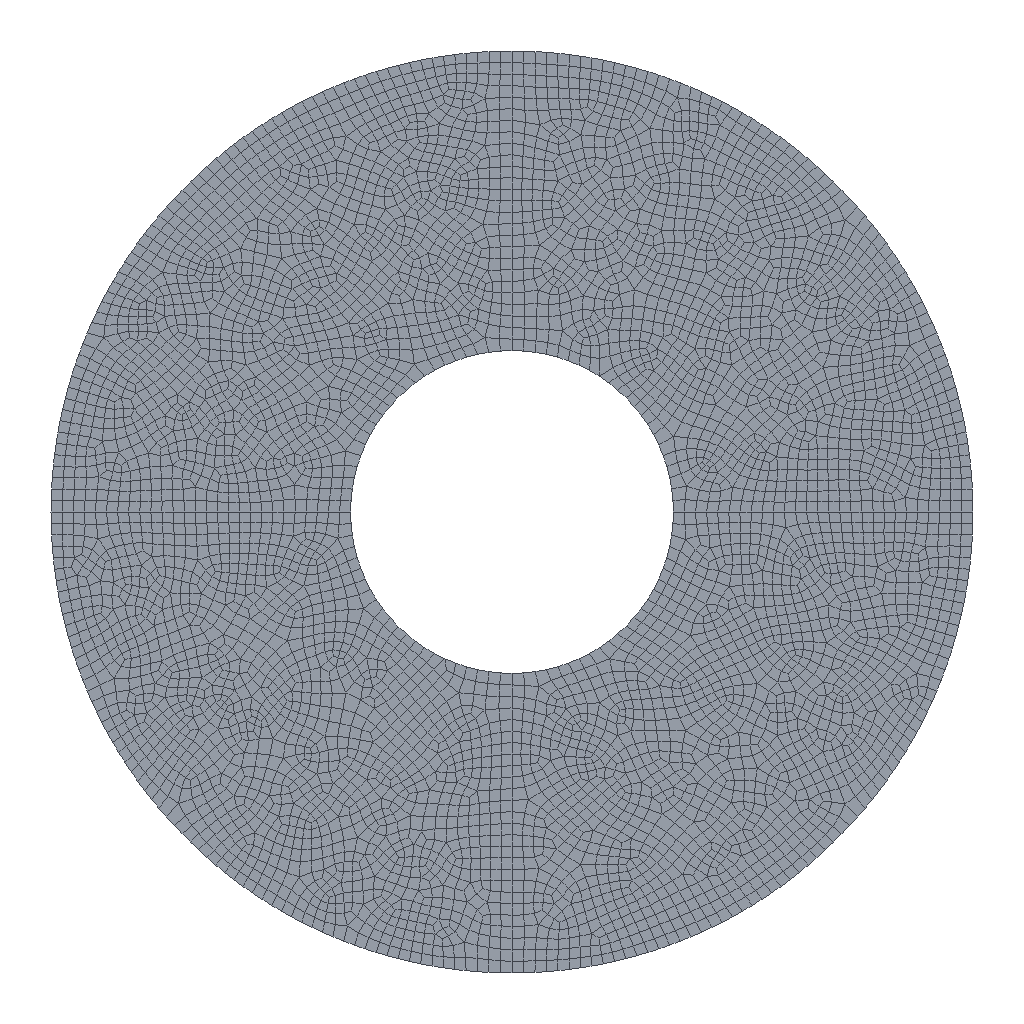Simulation study | abaqus
Set-up summary:
category,name,step,type,value,unit,region
solver,abaqus
solver,version,,,Abaqus/Standard 2020
units,not stated in the deck,,not stated
analysis,deck,,geostatic,geostatic; soils
load_step,Step-1,Step-1,geostatic,nlgeom=False
load_step,Step-2,Step-2,soils,nlgeom=True
contact,interactions,,,general=0 pairs=0 ties=0
load_step,requested,,,2
mesh,nodes,,,5893
mesh,elements,,,5609
element_type,CPE4RP,,plane,5503
element_type,COH2D4P,,cohesive,106
load,load commands in deck,,count,4
bc,support commands in deck,,count,2
material,BASE,,in results
material,MATERIAL-1,,in results
check,setup vs results,,match,"per instance, exact: element labels, types and connectivity; labels of the nodes the elements use; coordinates of those nodes at SINGLE_PRECISION in 1 of 1 instance(s)"
Abaqus input file, long lists of numbers shortened:
*Heading
** Job name: Job-1 Model name: Model-1
** Generated by: Abaqus/CAE 2020
*Preprint, echo=NO, model=NO, history=NO, contact=NO
**
** PARTS
**
*Part, name=Part-1
*Node
      1,           0.,         -20.
      2,           0.,          -7.
** (5891 more lines like these left out)
*Element, type=CPE4RP
   1,  141,  142,  707,  716
   2, 1011,  990,  980,  936
** (5501 more lines like these left out)
*Element, type=COH2D4P
5504, 5674, 5699,    8,  276, 5702, 5701
5505, 5675, 5674,  276,  275, 5703, 5702
** (104 more lines like these left out)
*Nset, nset=Set-19
    1,    2,    3,    4,    5,    6,    7,    8,    9,   10,   11,   12,   13,   14,   15,   16
   17,   18,   19,   20,   21,   22,   23,   24,   25,   26,   27,   28,   29,   30,   31,   32
** (360 more lines like these left out)
*Elset, elset=Set-19, generate
    1,  5503,     1
*Elset, elset=CohesiveSeam-2-Elements, generate
 5504,  5529,     1
*Nset, nset=CohesiveSeam-2-TopNodes
   7,   8, 252, 253, 254, 255, 256, 257, 258, 259, 260, 261, 262, 263, 264, 265
 266, 267, 268, 269, 270, 271, 272, 273, 274, 275, 276
*Nset, nset=CohesiveSeam-2-BottomNodes, generate
 5674,  5700,     1
*Nset, nset=CohesiveSeam-2-MidNodes, generate
 5701,  5727,     1
*Elset, elset=CohesiveSeam-3-Elements, generate
 5530,  5556,     1
*Nset, nset=CohesiveSeam-3-TopNodes
  3,  4, 55, 56, 57, 58, 59, 60, 61, 62, 63, 64, 65, 66, 67, 68
 69, 70, 71, 72, 73, 74, 75, 76, 77, 78, 79, 80
*Nset, nset=CohesiveSeam-3-BottomNodes, generate
 5728,  5755,     1
*Nset, nset=CohesiveSeam-3-MidNodes, generate
 5756,  5783,     1
*Elset, elset=CohesiveSeam-4-Elements, generate
 5557,  5582,     1
*Nset, nset=CohesiveSeam-4-TopNodes
  1,  2,  9, 10, 11, 12, 13, 14, 15, 16, 17, 18, 19, 20, 21, 22
 23, 24, 25, 26, 27, 28, 29, 30, 31, 32, 33
*Nset, nset=CohesiveSeam-4-BottomNodes, generate
 5784,  5810,     1
*Nset, nset=CohesiveSeam-4-MidNodes, generate
 5811,  5837,     1
*Elset, elset=CohesiveSeam-5-Elements, generate
 5583,  5609,     1
*Nset, nset=CohesiveSeam-5-TopNodes
   5,   6, 205, 206, 207, 208, 209, 210, 211, 212, 213, 214, 215, 216, 217, 218
 219, 220, 221, 222, 223, 224, 225, 226, 227, 228, 229, 230
*Nset, nset=CohesiveSeam-5-BottomNodes, generate
 5838,  5865,     1
*Nset, nset=CohesiveSeam-5-MidNodes, generate
 5866,  5893,     1
*Nset, nset=in2
 5727,
*Nset, nset=in3
 5783,
*Nset, nset=in4
 5811,
*Nset, nset=in5
 5866,
*Elset, elset=initial2, generate
 5526,  5529,     1
*Elset, elset=initial3, generate
 5553,  5556,     1
*Elset, elset=initial4, generate
 5557,  5560,     1
*Elset, elset=initial5, generate
 5583,  5585,     1
*Elset, elset=__PickedSurf7_S3, internal
   60,   75,   89,   90,  134,  149,  482,  483,  522, 5557, 5558, 5559, 5560, 5561, 5562, 5563
 5564, 5565, 5566, 5567, 5568, 5569, 5570, 5571, 5572, 5573, 5574, 5575, 5576, 5577, 5578, 5579
** (1 more lines like these left out)
*Elset, elset=__PickedSurf7_S1, internal
   55,   56,   57,  133,  151,  439,  480,  507,  509,  510,  511,  514,  516,  517,  518,  519
  524, 2829, 3207
*Elset, elset=__PickedSurf7_S4, internal
  470, 1561, 1565, 1583, 1599, 1600, 1875, 1877, 1879, 1880, 2795, 2826, 2845, 2851, 3209, 3213
 3214,
*Elset, elset=__PickedSurf7_S2, internal
 1495, 1497, 1512, 1523, 1560, 1584, 1585, 1874, 1890, 1892, 1893, 1895, 1898, 1900, 1903, 1905
 1907, 1908, 2776, 2797, 2808, 2825, 2830, 2849, 2850, 3309, 3311, 3313, 3315, 3318, 3319, 3320
** (1 more lines like these left out)
*Surface, type=ELEMENT, name=_PickedSurf7, internal
__PickedSurf7_S3, S3
__PickedSurf7_S1, S1
__PickedSurf7_S4, S4
__PickedSurf7_S2, S2
*Elset, elset=__PickedSurf19_S2, internal
 2776, 2797, 2808, 2825, 2830, 2849, 2850, 3309, 3311, 3313, 3315, 3318, 3319, 3320, 3321, 3324
 3326,
*Elset, elset=__PickedSurf19_S4, internal
 2795, 2826, 2845, 2851, 3209, 3213, 3214
*Elset, elset=__PickedSurf19_S1, internal
 2829, 3207
*Surface, type=ELEMENT, name=_PickedSurf19, internal
__PickedSurf19_S2, S2
__PickedSurf19_S4, S4
__PickedSurf19_S1, S1
*Elset, elset=__PickedSurf26_S1, internal
  55,  56,  57, 133, 151, 439, 480, 507, 509, 510, 511, 514, 516, 517, 518, 519
 524,
*Elset, elset=__PickedSurf26_S3, internal
  60,  75,  89,  90, 134, 149, 482, 483, 522
*Elset, elset=__PickedSurf26_S4, internal
 470,
*Surface, type=ELEMENT, name=_PickedSurf26, internal
__PickedSurf26_S1, S1
__PickedSurf26_S3, S3
__PickedSurf26_S4, S4
*Elset, elset=__PickedSurf33_S3, internal, generate
 5557,  5582,     1
*Surface, type=ELEMENT, name=_PickedSurf33, internal
__PickedSurf33_S3, S3
*Elset, elset=__PickedSurf40_S2, internal
 1495, 1497, 1512, 1523, 1560, 1584, 1585, 1874, 1890, 1892, 1893, 1895, 1898, 1900, 1903, 1905
 1907, 1908
*Elset, elset=__PickedSurf40_S4, internal
 1561, 1565, 1583, 1599, 1600, 1875, 1877, 1879, 1880
*Surface, type=ELEMENT, name=_PickedSurf40, internal
__PickedSurf40_S2, S2
__PickedSurf40_S4, S4
*Elset, elset=_CohesiveSeam-2-TopSurf_S3, internal, generate
 5504,  5529,     1
*Surface, type=ELEMENT, name=CohesiveSeam-2-TopSurf
_CohesiveSeam-2-TopSurf_S3, S3
*Elset, elset=_CohesiveSeam-2-BottomSurf_S1, internal, generate
 5504,  5529,     1
*Surface, type=ELEMENT, name=CohesiveSeam-2-BottomSurf
_CohesiveSeam-2-BottomSurf_S1, S1
*Elset, elset=_CohesiveSeam-3-TopSurf_S3, internal, generate
 5530,  5556,     1
*Surface, type=ELEMENT, name=CohesiveSeam-3-TopSurf
_CohesiveSeam-3-TopSurf_S3, S3
*Elset, elset=_CohesiveSeam-3-BottomSurf_S1, internal, generate
 5530,  5556,     1
*Surface, type=ELEMENT, name=CohesiveSeam-3-BottomSurf
_CohesiveSeam-3-BottomSurf_S1, S1
*Elset, elset=_CohesiveSeam-4-TopSurf_S3, internal, generate
 5557,  5582,     1
*Surface, type=ELEMENT, name=CohesiveSeam-4-TopSurf
_CohesiveSeam-4-TopSurf_S3, S3
*Elset, elset=_CohesiveSeam-4-BottomSurf_S1, internal, generate
 5557,  5582,     1
*Surface, type=ELEMENT, name=CohesiveSeam-4-BottomSurf
_CohesiveSeam-4-BottomSurf_S1, S1
*Elset, elset=_CohesiveSeam-5-TopSurf_S3, internal, generate
 5583,  5609,     1
*Surface, type=ELEMENT, name=CohesiveSeam-5-TopSurf
_CohesiveSeam-5-TopSurf_S3, S3
*Elset, elset=_CohesiveSeam-5-BottomSurf_S1, internal, generate
 5583,  5609,     1
*Surface, type=ELEMENT, name=CohesiveSeam-5-BottomSurf
_CohesiveSeam-5-BottomSurf_S1, S1
** Section: Section-base
*Solid Section, elset=Set-19, material=base
,
** Section: Section-coh
*Cohesive Section, elset=CohesiveSeam-2-Elements, controls=EC-1, material=Material-1, response=TRACTION SEPARATION
,
** Section: Section-coh
*Cohesive Section, elset=CohesiveSeam-3-Elements, controls=EC-1, material=Material-1, response=TRACTION SEPARATION
,
** Section: Section-coh
*Cohesive Section, elset=CohesiveSeam-4-Elements, controls=EC-1, material=Material-1, response=TRACTION SEPARATION
,
** Section: Section-coh
*Cohesive Section, elset=CohesiveSeam-5-Elements, controls=EC-1, material=Material-1, response=TRACTION SEPARATION
,
*End Part
**
**
** ASSEMBLY
**
*Assembly, name=Assembly
**
*Instance, name=Part-1-1, part=Part-1
*End Instance
**
*Nset, nset=Set-1, instance=Part-1-1
    1,    2,    3,    4,    5,    6,    7,    8,    9,   10,   11,   12,   13,   14,   15,   16
   17,   18,   19,   20,   21,   22,   23,   24,   25,   26,   27,   28,   29,   30,   31,   32
** (360 more lines like these left out)
*Elset, elset=Set-1, instance=Part-1-1, generate
    1,  5609,     1
*Nset, nset=Set-2, instance=Part-1-1
    1,    2,    3,    4,    5,    6,    7,    8,    9,   10,   11,   12,   13,   14,   15,   16
   17,   18,   19,   20,   21,   22,   23,   24,   25,   26,   27,   28,   29,   30,   31,   32
** (360 more lines like these left out)
*Elset, elset=Set-2, instance=Part-1-1, generate
    1,  5503,     1
*Nset, nset=Set-3, instance=Part-1-1
    1,    4,    5,    8,   81,   82,   83,   84,   85,   86,   87,   88,   89,   90,   91,   92
   93,   94,   95,   96,   97,   98,   99,  100,  101,  102,  103,  104,  105,  106,  107,  108
** (14 more lines like these left out)
*Elset, elset=Set-3, instance=Part-1-1
    1,   17,   33,   34,   35,  152,  166,  168,  169,  181,  182,  183,  184,  193,  194,  197
  200,  203,  207,  208,  209,  210,  211,  213,  214,  274,  308,  354,  464,  480,  487,  490
** (14 more lines like these left out)
*Nset, nset=Set-4, instance=Part-1-1
    2,    3,    6,    7,   34,   35,   36,   37,   38,   39,   40,   41,   42,   43,   44,   45
   46,   47,   48,   49,   50,   51,   52,   53,   54,  231,  232,  233,  234,  235,  236,  237
** (4 more lines like these left out)
*Elset, elset=Set-4, instance=Part-1-1
  101,  103,  118,  126,  127,  128,  130,  145,  423,  457,  465,  470,  471,  472,  473,  474
  475,  476,  477,  478,  479,  568, 1386, 1406, 1409, 1601, 1610, 1611, 1626, 1627, 1639, 1714
** (4 more lines like these left out)
*Nset, nset=Set-5, instance=Part-1-1
    1,    4,    5,    8,   81,   82,   83,   84,   85,   86,   87,   88,   89,   90,   91,   92
   93,   94,   95,   96,   97,   98,   99,  100,  101,  102,  103,  104,  105,  106,  107,  108
** (14 more lines like these left out)
*Elset, elset=Set-5, instance=Part-1-1
    1,   17,   33,   34,   35,  152,  166,  168,  169,  181,  182,  183,  184,  193,  194,  197
  200,  203,  207,  208,  209,  210,  211,  213,  214,  274,  308,  354,  464,  480,  487,  490
** (14 more lines like these left out)
*Nset, nset=Set-6, instance=Part-1-1
    1,    4,    5,    8, 5699, 5754, 5810, 5865
*Nset, nset=Set-7, instance=Part-1-1
   1,   4,  81,  82,  83,  84,  85,  86,  87,  88,  89,  90,  91,  92,  93,  94
  95,  96,  97,  98,  99, 100, 101, 102, 103, 104, 105, 106, 107, 108, 109, 110
** (2 more lines like these left out)
*Elset, elset=Set-7, instance=Part-1-1
   1,  17,  33,  34,  35, 152, 166, 168, 169, 181, 182, 183, 184, 193, 194, 197
 200, 203, 207, 208, 209, 210, 211, 213, 214, 274, 308, 354, 464, 480, 487, 490
** (2 more lines like these left out)
*Nset, nset=Set-8, instance=Part-1-1
    1,    2,    3,    4,    5,    6,    7,    8,    9,   10,   11,   12,   13,   14,   15,   16
   17,   18,   19,   20,   21,   22,   23,   24,   25,   26,   27,   28,   29,   30,   31,   32
** (12 more lines like these left out)
*Elset, elset=Set-8, instance=Part-1-1
   55,   56,   57,   60,   75,   89,   90,  133,  134,  149,  151,  439,  470,  480,  482,  483
  507,  509,  510,  511,  514,  516,  517,  518,  519,  522,  524, 1495, 1497, 1512, 1523, 1560
** (10 more lines like these left out)
*End Assembly
**
** ELEMENT CONTROLS
**
*Section Controls, name=EC-1, ELEMENT DELETION=YES
1., 1., 1.
*Amplitude, name=Amp-1
             0.,              0.,             50.,              1.
**
** MATERIALS
**
*Material, name=Material-1
*Damage Initiation, criterion=MAXS
 1e+06, 1e+06, 1e+06
*Damage Evolution, type=DISPLACEMENT
 1e-12,
*Elastic, type=TRACTION
 1.5e+10, 1.5e+10, 1.5e+10
*Gap Flow
 0.001,
*Material, name=base
*Elastic
 1.5e+10, 0.25
*Permeability, specific=9800.
 1e-07, 0.2
**
** PREDEFINED FIELDS
**
** Name: Predefined Field-1   Type: Void ratio
*Initial Conditions, TYPE=RATIO
Set-1, 0.2
** Name: Predefined Field-2   Type: Stress
*Initial Conditions, type=STRESS
Set-2, -1e+06, -1e+06, -1e+06, 0.,
** ----------------------------------------------------------------
*initial conditions,type=initial gap
Part-1-1.initial2
*initial conditions,type=initial gap
Part-1-1.initial3
*initial conditions,type=initial gap
Part-1-1.initial4
*initial conditions,type=initial gap
Part-1-1.initial5
**
** STEP: Step-1
**
*Step, name=Step-1, nlgeom=NO, unsymm=YES
*Geostatic
**
** BOUNDARY CONDITIONS
**
** Name: BC-1 Type: 位移/转角
*Boundary
Set-3, 1, 1
Set-3, 2, 2
**
** OUTPUT REQUESTS
**
*Restart, write, frequency=0
**
** FIELD OUTPUT: F-Output-1
**
*Output, field
*Node Output
CF, POR, RF, U, V
*Element Output, directions=YES
CFAILURE, E, FLUVR, FLVEL, LE, MISES, MISESMAX, MISESONLY, NE, PE, PEEQ, PEEQT, PEMAG, PRESSONLY, S, SAT
SDEG, SEQUT, SROCK, VEEQ, VOIDR, YIELDPOT
*Contact Output
CDISP, CSTRESS
**
** HISTORY OUTPUT: H-Output-1
**
*Output, history, variable=PRESELECT
*End Step
** ----------------------------------------------------------------
**
** STEP: Step-2
**
*Step, name=Step-2, nlgeom=YES, inc=1000, unsymm=YES
*Soils, consolidation, end=PERIOD, utol=1e+29, creep=none
0.1, 100., 1e-05, 1.,
**
** LOADS
**
** Name: Load-1   Type: Concentrated pore fluid
*Cflow
Part-1-1.in2,  , -0.001
** Name: Load-2   Type: Concentrated pore fluid
*Cflow
Part-1-1.in3,  , -0.001
** Name: Load-3   Type: Concentrated pore fluid
*Cflow
Part-1-1.in4,  , -0.001
** Name: Load-4   Type: Concentrated pore fluid
*Cflow
Part-1-1.in5,  , -0.001
**
** CONTROLS
**
*Controls, reset
*Controls, parameters=time incrementation
, , , , , , , 15, , ,
**
** OUTPUT REQUESTS
**
*Restart, write, frequency=0
**
** FIELD OUTPUT: F-Output-1
**
*Output, field
*Node Output
CF, POR, RF, U, V
*Element Output, directions=YES
CFAILURE, E, FLUVR, FLVEL, LE, MISES, MISESMAX, MISESONLY, NE, PE, PEEQ, PEEQT, PEMAG, PRESSONLY, S, SAT
SDEG, SEQUT, SROCK, VEEQ, VOIDR, YIELDPOT,pfopen
*Contact Output
CDISP, CSTRESS
**
** HISTORY OUTPUT: H-Output-1
**
*Output, history, variable=PRESELECT
*End Step
Results summary:
result,step,,completed,increments=1 time=1.0/1.0
result,step,,completed,increments=107 time=100.0/100.0
result,analysis,,,"soils, consolidation"
result,last_loadstep,,,2
result,analysis steps,,count,2
result,primary field,,,"U, POR"
result,reaction total,,FX,-0.75,model units
result,reaction total,,FY,-3.25,model units
result,reaction total,,FZ,0.0,model units